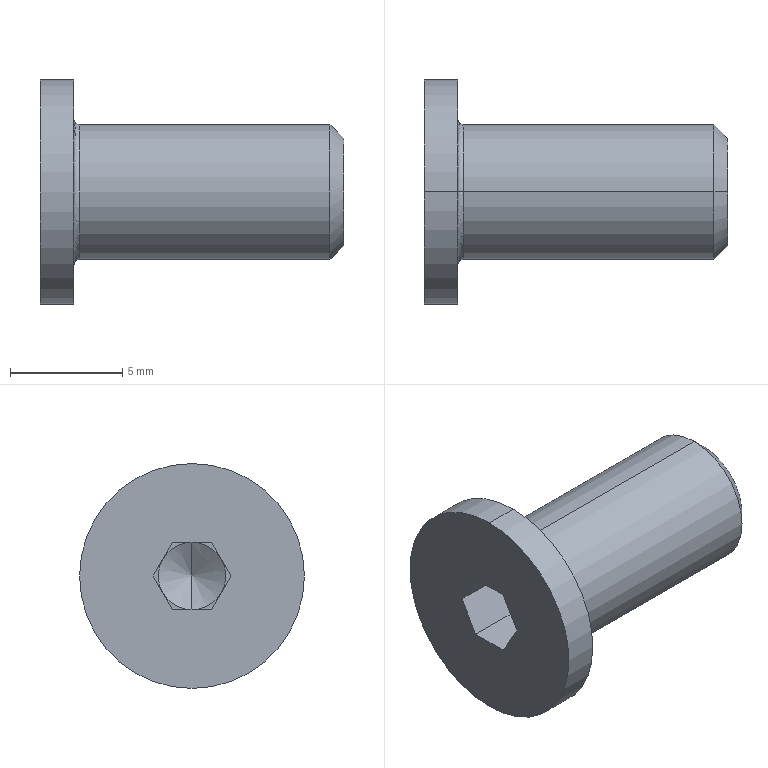Part | STEP file | cbss6_12_2_03 | 1 solid | 25 faces | box 13.5 x 10 x 10 mm | volume 420.837 mm3 | plane 15 | cylinder 4 | cone 4 | spline 2 | commonest cylinder face diameters 6 x2 10 x2